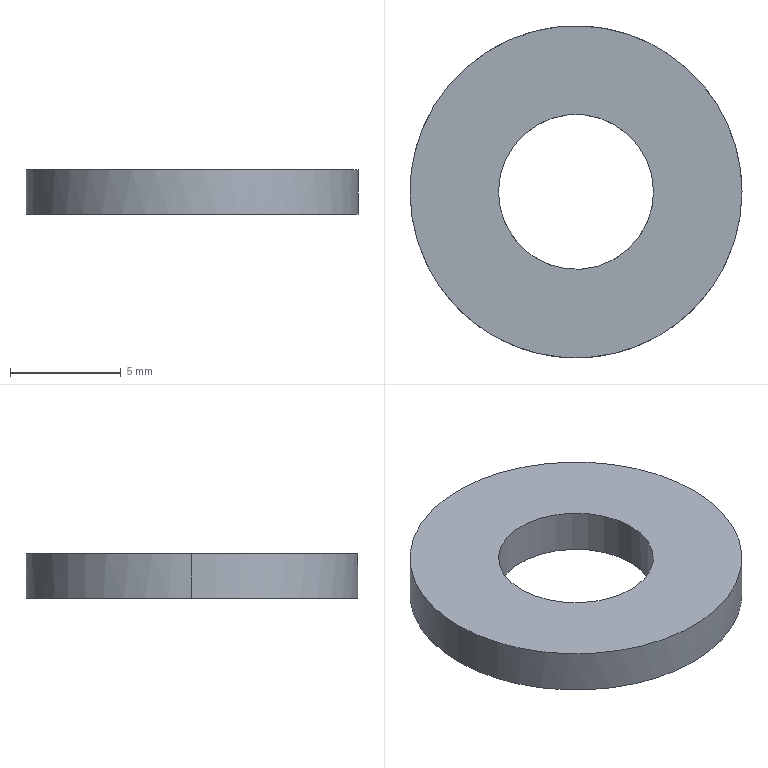Part | STEP file | Positioning_id2198_x_t | 1 solid | 6 faces | box 15 x 15 x 2 mm | volume 276.46 mm3 | cylinder 4 | plane 2 | commonest cylinder face diameters 7 x2 15 x2
STEP:
#1=CARTESIAN_POINT('',(0.,0.,0.));
#2=DIRECTION('',(0.,0.,1.));
#3=DIRECTION('',(1.,0.,0.));
#4=AXIS2_PLACEMENT_3D('',#1,#2,#3);
#5=CARTESIAN_POINT('',(-999.002,416.,33.5));
#6=VERTEX_POINT('',#5);
#7=CARTESIAN_POINT('',(-1006.002,416.,33.5));
#8=VERTEX_POINT('',#7);
#9=CARTESIAN_POINT('',(-1002.502,416.,33.5));
#10=DIRECTION('',(0.,0.,1.));
#11=DIRECTION('',(0.,1.,0.));
#12=AXIS2_PLACEMENT_3D('',#9,#10,#11);
#13=CIRCLE('',#12,3.5);
#14=CARTESIAN_POINT('',(-1002.502,416.,30.5));
#15=DIRECTION('',(0.,0.,-1.));
#16=DIRECTION('',(-1.,0.,0.));
#17=AXIS2_PLACEMENT_3D('',#14,#15,#16);
#18=CYLINDRICAL_SURFACE('',#17,3.5);
#19=CARTESIAN_POINT('',(7.854,-3.));
#20=DIRECTION('',(-1.,0.));
#21=VECTOR('',#20,1.);
#22=LINE('',#19,#21);
#23=(GEOMETRIC_REPRESENTATION_CONTEXT(2)PARAMETRIC_REPRESENTATION_CONTEXT()REPRESENTATION_CONTEXT('',''));
#24=DEFINITIONAL_REPRESENTATION('',(#22),#23);
#25=PCURVE('',#18,#24);
#26=CARTESIAN_POINT('',(-1002.502,416.,33.5));
#27=DIRECTION('',(0.,0.,1.));
#28=DIRECTION('',(-1.,0.,0.));
#29=AXIS2_PLACEMENT_3D('',#26,#27,#28);
#30=PLANE('',#29);
#31=CARTESIAN_POINT('',(0.,0.));
#32=DIRECTION('',(0.,-1.));
#33=AXIS2_PLACEMENT_2D('',#31,#32);
#34=CIRCLE('',#33,3.5);
#35=(GEOMETRIC_REPRESENTATION_CONTEXT(2)PARAMETRIC_REPRESENTATION_CONTEXT()REPRESENTATION_CONTEXT('',''));
#36=DEFINITIONAL_REPRESENTATION('',(#34),#35);
#37=PCURVE('',#30,#36);
#38=SURFACE_CURVE('',#13,(#25,#37),.PCURVE_S1.);
#39=EDGE_CURVE('',#6,#8,#38,.T.);
#40=ORIENTED_EDGE('',*,*,#39,.F.);
#41=CARTESIAN_POINT('',(-999.002,416.,31.5));
#42=VERTEX_POINT('',#41);
#43=CARTESIAN_POINT('',(-999.002,416.,31.5));
#44=DIRECTION('',(0.,0.,1.));
#45=VECTOR('',#44,1.);
#46=LINE('',#43,#45);
#47=CARTESIAN_POINT('',(3.142,-1.));
#48=DIRECTION('',(0.,-1.));
#49=VECTOR('',#48,1.);
#50=LINE('',#47,#49);
#51=(GEOMETRIC_REPRESENTATION_CONTEXT(2)PARAMETRIC_REPRESENTATION_CONTEXT()REPRESENTATION_CONTEXT('',''));
#52=DEFINITIONAL_REPRESENTATION('',(#50),#51);
#53=PCURVE('',#18,#52);
#54=CARTESIAN_POINT('',(-1002.502,416.,30.5));
#55=DIRECTION('',(0.,0.,-1.));
#56=DIRECTION('',(-1.,0.,0.));
#57=AXIS2_PLACEMENT_3D('',#54,#55,#56);
#58=CYLINDRICAL_SURFACE('',#57,3.5);
#59=CARTESIAN_POINT('',(3.142,-1.));
#60=DIRECTION('',(0.,-1.));
#61=VECTOR('',#60,1.);
#62=LINE('',#59,#61);
#63=(GEOMETRIC_REPRESENTATION_CONTEXT(2)PARAMETRIC_REPRESENTATION_CONTEXT()REPRESENTATION_CONTEXT('',''));
#64=DEFINITIONAL_REPRESENTATION('',(#62),#63);
#65=PCURVE('',#58,#64);
#66=SURFACE_CURVE('',#46,(#53,#65),.PCURVE_S1.);
#67=EDGE_CURVE('',#42,#6,#66,.T.);
#68=ORIENTED_EDGE('',*,*,#67,.F.);
#69=CARTESIAN_POINT('',(-1006.002,416.,31.5));
#70=VERTEX_POINT('',#69);
#71=CARTESIAN_POINT('',(-1002.502,416.,31.5));
#72=DIRECTION('',(0.,0.,-1.));
#73=DIRECTION('',(0.,1.,0.));
#74=AXIS2_PLACEMENT_3D('',#71,#72,#73);
#75=CIRCLE('',#74,3.5);
#76=CARTESIAN_POINT('',(-4.712,-1.));
#77=DIRECTION('',(1.,0.));
#78=VECTOR('',#77,1.);
#79=LINE('',#76,#78);
#80=(GEOMETRIC_REPRESENTATION_CONTEXT(2)PARAMETRIC_REPRESENTATION_CONTEXT()REPRESENTATION_CONTEXT('',''));
#81=DEFINITIONAL_REPRESENTATION('',(#79),#80);
#82=PCURVE('',#18,#81);
#83=CARTESIAN_POINT('',(-1002.502,416.,31.5));
#84=DIRECTION('',(0.,0.,-1.));
#85=DIRECTION('',(1.,0.,0.));
#86=AXIS2_PLACEMENT_3D('',#83,#84,#85);
#87=PLANE('',#86);
#88=CARTESIAN_POINT('',(0.,0.));
#89=DIRECTION('',(0.,-1.));
#90=AXIS2_PLACEMENT_2D('',#88,#89);
#91=CIRCLE('',#90,3.5);
#92=(GEOMETRIC_REPRESENTATION_CONTEXT(2)PARAMETRIC_REPRESENTATION_CONTEXT()REPRESENTATION_CONTEXT('',''));
#93=DEFINITIONAL_REPRESENTATION('',(#91),#92);
#94=PCURVE('',#87,#93);
#95=SURFACE_CURVE('',#75,(#82,#94),.PCURVE_S1.);
#96=EDGE_CURVE('',#70,#42,#95,.T.);
#97=ORIENTED_EDGE('',*,*,#96,.F.);
#98=CARTESIAN_POINT('',(-1006.002,416.,31.5));
#99=DIRECTION('',(0.,0.,-1.));
#100=VECTOR('',#99,1.);
#101=LINE('',#98,#100);
#102=CARTESIAN_POINT('',(0.,-1.));
#103=DIRECTION('',(0.,1.));
#104=VECTOR('',#103,1.);
#105=LINE('',#102,#104);
#106=(GEOMETRIC_REPRESENTATION_CONTEXT(2)PARAMETRIC_REPRESENTATION_CONTEXT()REPRESENTATION_CONTEXT('',''));
#107=DEFINITIONAL_REPRESENTATION('',(#105),#106);
#108=PCURVE('',#18,#107);
#109=CARTESIAN_POINT('',(6.283,-1.));
#110=DIRECTION('',(0.,1.));
#111=VECTOR('',#110,1.);
#112=LINE('',#109,#111);
#113=(GEOMETRIC_REPRESENTATION_CONTEXT(2)PARAMETRIC_REPRESENTATION_CONTEXT()REPRESENTATION_CONTEXT('',''));
#114=DEFINITIONAL_REPRESENTATION('',(#112),#113);
#115=PCURVE('',#58,#114);
#116=SURFACE_CURVE('',#101,(#108,#115),.PCURVE_S1.);
#117=EDGE_CURVE('',#8,#70,#116,.T.);
#118=ORIENTED_EDGE('',*,*,#117,.F.);
#119=EDGE_LOOP('',(#40,#68,#97,#118));
#120=FACE_BOUND('',#119,.F.);
#121=ADVANCED_FACE('',(#120),#18,.F.);
#122=CARTESIAN_POINT('',(-1010.002,416.,31.5));
#123=VERTEX_POINT('',#122);
#124=CARTESIAN_POINT('',(-1010.002,416.,33.5));
#125=VERTEX_POINT('',#124);
#126=CARTESIAN_POINT('',(-1010.002,416.,31.5));
#127=DIRECTION('',(0.,0.,1.));
#128=VECTOR('',#127,1.);
#129=LINE('',#126,#128);
#130=CARTESIAN_POINT('',(-1002.502,416.,30.5));
#131=DIRECTION('',(0.,0.,-1.));
#132=DIRECTION('',(-1.,0.,0.));
#133=AXIS2_PLACEMENT_3D('',#130,#131,#132);
#134=CYLINDRICAL_SURFACE('',#133,7.5);
#135=CARTESIAN_POINT('',(6.283,-1.));
#136=DIRECTION('',(0.,-1.));
#137=VECTOR('',#136,1.);
#138=LINE('',#135,#137);
#139=(GEOMETRIC_REPRESENTATION_CONTEXT(2)PARAMETRIC_REPRESENTATION_CONTEXT()REPRESENTATION_CONTEXT('',''));
#140=DEFINITIONAL_REPRESENTATION('',(#138),#139);
#141=PCURVE('',#134,#140);
#142=CARTESIAN_POINT('',(-1002.502,416.,30.5));
#143=DIRECTION('',(0.,0.,-1.));
#144=DIRECTION('',(-1.,0.,0.));
#145=AXIS2_PLACEMENT_3D('',#142,#143,#144);
#146=CYLINDRICAL_SURFACE('',#145,7.5);
#147=CARTESIAN_POINT('',(0.,-1.));
#148=DIRECTION('',(0.,-1.));
#149=VECTOR('',#148,1.);
#150=LINE('',#147,#149);
#151=(GEOMETRIC_REPRESENTATION_CONTEXT(2)PARAMETRIC_REPRESENTATION_CONTEXT()REPRESENTATION_CONTEXT('',''));
#152=DEFINITIONAL_REPRESENTATION('',(#150),#151);
#153=PCURVE('',#146,#152);
#154=SURFACE_CURVE('',#129,(#141,#153),.PCURVE_S1.);
#155=EDGE_CURVE('',#123,#125,#154,.T.);
#156=ORIENTED_EDGE('',*,*,#155,.F.);
#157=CARTESIAN_POINT('',(-1002.502,408.5,31.5));
#158=VERTEX_POINT('',#157);
#159=CARTESIAN_POINT('',(-1002.502,416.,31.5));
#160=DIRECTION('',(0.,0.,-1.));
#161=DIRECTION('',(0.,1.,0.));
#162=AXIS2_PLACEMENT_3D('',#159,#160,#161);
#163=CIRCLE('',#162,7.5);
#164=CARTESIAN_POINT('',(1.571,-1.));
#165=DIRECTION('',(1.,0.));
#166=VECTOR('',#165,1.);
#167=LINE('',#164,#166);
#168=(GEOMETRIC_REPRESENTATION_CONTEXT(2)PARAMETRIC_REPRESENTATION_CONTEXT()REPRESENTATION_CONTEXT('',''));
#169=DEFINITIONAL_REPRESENTATION('',(#167),#168);
#170=PCURVE('',#134,#169);
#171=CARTESIAN_POINT('',(0.,0.));
#172=DIRECTION('',(0.,-1.));
#173=AXIS2_PLACEMENT_2D('',#171,#172);
#174=CIRCLE('',#173,7.5);
#175=(GEOMETRIC_REPRESENTATION_CONTEXT(2)PARAMETRIC_REPRESENTATION_CONTEXT()REPRESENTATION_CONTEXT('',''));
#176=DEFINITIONAL_REPRESENTATION('',(#174),#175);
#177=PCURVE('',#87,#176);
#178=SURFACE_CURVE('',#163,(#170,#177),.PCURVE_S1.);
#179=EDGE_CURVE('',#158,#123,#178,.T.);
#180=ORIENTED_EDGE('',*,*,#179,.F.);
#181=CARTESIAN_POINT('',(-995.002,416.,31.5));
#182=VERTEX_POINT('',#181);
#183=CARTESIAN_POINT('',(-1002.502,416.,31.5));
#184=DIRECTION('',(0.,0.,-1.));
#185=DIRECTION('',(0.,1.,0.));
#186=AXIS2_PLACEMENT_3D('',#183,#184,#185);
#187=CIRCLE('',#186,7.5);
#188=CARTESIAN_POINT('',(1.571,-1.));
#189=DIRECTION('',(1.,0.));
#190=VECTOR('',#189,1.);
#191=LINE('',#188,#190);
#192=(GEOMETRIC_REPRESENTATION_CONTEXT(2)PARAMETRIC_REPRESENTATION_CONTEXT()REPRESENTATION_CONTEXT('',''));
#193=DEFINITIONAL_REPRESENTATION('',(#191),#192);
#194=PCURVE('',#134,#193);
#195=CARTESIAN_POINT('',(0.,0.));
#196=DIRECTION('',(0.,-1.));
#197=AXIS2_PLACEMENT_2D('',#195,#196);
#198=CIRCLE('',#197,7.5);
#199=(GEOMETRIC_REPRESENTATION_CONTEXT(2)PARAMETRIC_REPRESENTATION_CONTEXT()REPRESENTATION_CONTEXT('',''));
#200=DEFINITIONAL_REPRESENTATION('',(#198),#199);
#201=PCURVE('',#87,#200);
#202=SURFACE_CURVE('',#187,(#194,#201),.PCURVE_S1.);
#203=EDGE_CURVE('',#182,#158,#202,.T.);
#204=ORIENTED_EDGE('',*,*,#203,.F.);
#205=CARTESIAN_POINT('',(-995.002,416.,33.5));
#206=VERTEX_POINT('',#205);
#207=CARTESIAN_POINT('',(-995.002,416.,31.5));
#208=DIRECTION('',(0.,0.,-1.));
#209=VECTOR('',#208,1.);
#210=LINE('',#207,#209);
#211=CARTESIAN_POINT('',(3.142,-1.));
#212=DIRECTION('',(0.,1.));
#213=VECTOR('',#212,1.);
#214=LINE('',#211,#213);
#215=(GEOMETRIC_REPRESENTATION_CONTEXT(2)PARAMETRIC_REPRESENTATION_CONTEXT()REPRESENTATION_CONTEXT('',''));
#216=DEFINITIONAL_REPRESENTATION('',(#214),#215);
#217=PCURVE('',#134,#216);
#218=CARTESIAN_POINT('',(3.142,-1.));
#219=DIRECTION('',(0.,1.));
#220=VECTOR('',#219,1.);
#221=LINE('',#218,#220);
#222=(GEOMETRIC_REPRESENTATION_CONTEXT(2)PARAMETRIC_REPRESENTATION_CONTEXT()REPRESENTATION_CONTEXT('',''));
#223=DEFINITIONAL_REPRESENTATION('',(#221),#222);
#224=PCURVE('',#146,#223);
#225=SURFACE_CURVE('',#210,(#217,#224),.PCURVE_S1.);
#226=EDGE_CURVE('',#206,#182,#225,.T.);
#227=ORIENTED_EDGE('',*,*,#226,.F.);
#228=CARTESIAN_POINT('',(-1002.502,416.,33.5));
#229=DIRECTION('',(0.,0.,1.));
#230=DIRECTION('',(0.,1.,0.));
#231=AXIS2_PLACEMENT_3D('',#228,#229,#230);
#232=CIRCLE('',#231,7.5);
#233=CARTESIAN_POINT('',(7.854,-3.));
#234=DIRECTION('',(-1.,0.));
#235=VECTOR('',#234,1.);
#236=LINE('',#233,#235);
#237=(GEOMETRIC_REPRESENTATION_CONTEXT(2)PARAMETRIC_REPRESENTATION_CONTEXT()REPRESENTATION_CONTEXT('',''));
#238=DEFINITIONAL_REPRESENTATION('',(#236),#237);
#239=PCURVE('',#134,#238);
#240=CARTESIAN_POINT('',(0.,0.));
#241=DIRECTION('',(0.,-1.));
#242=AXIS2_PLACEMENT_2D('',#240,#241);
#243=CIRCLE('',#242,7.5);
#244=(GEOMETRIC_REPRESENTATION_CONTEXT(2)PARAMETRIC_REPRESENTATION_CONTEXT()REPRESENTATION_CONTEXT('',''));
#245=DEFINITIONAL_REPRESENTATION('',(#243),#244);
#246=PCURVE('',#30,#245);
#247=SURFACE_CURVE('',#232,(#239,#246),.PCURVE_S1.);
#248=EDGE_CURVE('',#125,#206,#247,.T.);
#249=ORIENTED_EDGE('',*,*,#248,.F.);
#250=EDGE_LOOP('',(#156,#180,#204,#227,#249));
#251=FACE_BOUND('',#250,.T.);
#252=ADVANCED_FACE('',(#251),#134,.T.);
#253=CARTESIAN_POINT('',(-1002.502,412.5,31.5));
#254=VERTEX_POINT('',#253);
#255=CARTESIAN_POINT('',(-999.002,416.,31.5));
#256=CARTESIAN_POINT('',(-999.002,412.5,31.5));
#257=CARTESIAN_POINT('',(-1002.502,412.5,31.5));
#258=(BOUNDED_CURVE()B_SPLINE_CURVE(2,(#255,#256,#257),.UNSPECIFIED.,.F.,.F.)B_SPLINE_CURVE_WITH_KNOTS((3,3),(0.,1.),.PIECEWISE_BEZIER_KNOTS.)CURVE()GEOMETRIC_REPRESENTATION_ITEM()RATIONAL_B_SPLINE_CURVE((1.,0.7071,1.))REPRESENTATION_ITEM(''));
#259=CARTESIAN_POINT('',(3.5,0.));
#260=CARTESIAN_POINT('',(3.5,3.5));
#261=CARTESIAN_POINT('',(0.,3.5));
#262=(BOUNDED_CURVE()B_SPLINE_CURVE(2,(#259,#260,#261),.UNSPECIFIED.,.F.,.F.)B_SPLINE_CURVE_WITH_KNOTS((3,3),(0.,1.),.PIECEWISE_BEZIER_KNOTS.)CURVE()GEOMETRIC_REPRESENTATION_ITEM()RATIONAL_B_SPLINE_CURVE((1.,0.7071,1.))REPRESENTATION_ITEM(''));
#263=(GEOMETRIC_REPRESENTATION_CONTEXT(2)PARAMETRIC_REPRESENTATION_CONTEXT()REPRESENTATION_CONTEXT('',''));
#264=DEFINITIONAL_REPRESENTATION('',(#262),#263);
#265=PCURVE('',#87,#264);
#266=CARTESIAN_POINT('',(3.142,-1.));
#267=CARTESIAN_POINT('',(3.163,-1.));
#268=CARTESIAN_POINT('',(3.206,-1.));
#269=CARTESIAN_POINT('',(3.273,-1.));
#270=CARTESIAN_POINT('',(3.342,-1.));
#271=CARTESIAN_POINT('',(3.411,-1.));
#272=CARTESIAN_POINT('',(3.482,-1.));
#273=CARTESIAN_POINT('',(3.555,-1.));
#274=CARTESIAN_POINT('',(3.628,-1.));
#275=CARTESIAN_POINT('',(3.702,-1.));
#276=CARTESIAN_POINT('',(3.777,-1.));
#277=CARTESIAN_POINT('',(3.852,-1.));
#278=CARTESIAN_POINT('',(3.927,-1.));
#279=CARTESIAN_POINT('',(4.002,-1.));
#280=CARTESIAN_POINT('',(4.077,-1.));
#281=CARTESIAN_POINT('',(4.152,-1.));
#282=CARTESIAN_POINT('',(4.226,-1.));
#283=CARTESIAN_POINT('',(4.299,-1.));
#284=CARTESIAN_POINT('',(4.372,-1.));
#285=CARTESIAN_POINT('',(4.443,-1.));
#286=CARTESIAN_POINT('',(4.512,-1.));
#287=CARTESIAN_POINT('',(4.581,-1.));
#288=CARTESIAN_POINT('',(4.648,-1.));
#289=CARTESIAN_POINT('',(4.691,-1.));
#290=CARTESIAN_POINT('',(4.712,-1.));
#291=B_SPLINE_CURVE_WITH_KNOTS('',3,(#266,#267,#268,#269,#270,#271,#272,#273,#274,#275,#276,#277,#278,#279,#280,#281,#282,#283,#284,#285,#286,#287,#288,#289,#290),.UNSPECIFIED.,.F.,.F.,(4,1,1,1,1,1,1,1,1,1,1,1,1,1,1,1,1,1,1,1,1,1,4),(0.,0.04545,0.09091,0.1364,0.1818,0.2273,0.2727,0.3182,0.3636,0.4091,0.4545,0.5,0.5455,0.5909,0.6364,0.6818,0.7273,0.7727,0.8182,0.8636,0.9091,0.9545,1.),.QUASI_UNIFORM_KNOTS.);
#292=(GEOMETRIC_REPRESENTATION_CONTEXT(2)PARAMETRIC_REPRESENTATION_CONTEXT()REPRESENTATION_CONTEXT('',''));
#293=DEFINITIONAL_REPRESENTATION('',(#291),#292);
#294=PCURVE('',#58,#293);
#295=SURFACE_CURVE('',#258,(#265,#294),.PCURVE_S1.);
#296=EDGE_CURVE('',#42,#254,#295,.T.);
#297=ORIENTED_EDGE('',*,*,#296,.F.);
#298=ORIENTED_EDGE('',*,*,#96,.F.);
#299=CARTESIAN_POINT('',(-1002.502,412.5,31.5));
#300=CARTESIAN_POINT('',(-1006.002,412.5,31.5));
#301=CARTESIAN_POINT('',(-1006.002,416.,31.5));
#302=(BOUNDED_CURVE()B_SPLINE_CURVE(2,(#299,#300,#301),.UNSPECIFIED.,.F.,.F.)B_SPLINE_CURVE_WITH_KNOTS((3,3),(0.,1.),.PIECEWISE_BEZIER_KNOTS.)CURVE()GEOMETRIC_REPRESENTATION_ITEM()RATIONAL_B_SPLINE_CURVE((1.,0.7071,1.))REPRESENTATION_ITEM(''));
#303=CARTESIAN_POINT('',(0.,3.5));
#304=CARTESIAN_POINT('',(-3.5,3.5));
#305=CARTESIAN_POINT('',(-3.5,0.));
#306=(BOUNDED_CURVE()B_SPLINE_CURVE(2,(#303,#304,#305),.UNSPECIFIED.,.F.,.F.)B_SPLINE_CURVE_WITH_KNOTS((3,3),(0.,1.),.PIECEWISE_BEZIER_KNOTS.)CURVE()GEOMETRIC_REPRESENTATION_ITEM()RATIONAL_B_SPLINE_CURVE((1.,0.7071,1.))REPRESENTATION_ITEM(''));
#307=(GEOMETRIC_REPRESENTATION_CONTEXT(2)PARAMETRIC_REPRESENTATION_CONTEXT()REPRESENTATION_CONTEXT('',''));
#308=DEFINITIONAL_REPRESENTATION('',(#306),#307);
#309=PCURVE('',#87,#308);
#310=CARTESIAN_POINT('',(4.712,-1.));
#311=CARTESIAN_POINT('',(4.734,-1.));
#312=CARTESIAN_POINT('',(4.777,-1.));
#313=CARTESIAN_POINT('',(4.844,-1.));
#314=CARTESIAN_POINT('',(4.912,-1.));
#315=CARTESIAN_POINT('',(4.982,-1.));
#316=CARTESIAN_POINT('',(5.053,-1.));
#317=CARTESIAN_POINT('',(5.125,-1.));
#318=CARTESIAN_POINT('',(5.199,-1.));
#319=CARTESIAN_POINT('',(5.273,-1.));
#320=CARTESIAN_POINT('',(5.347,-1.));
#321=CARTESIAN_POINT('',(5.422,-1.));
#322=CARTESIAN_POINT('',(5.498,-1.));
#323=CARTESIAN_POINT('',(5.573,-1.));
#324=CARTESIAN_POINT('',(5.648,-1.));
#325=CARTESIAN_POINT('',(5.723,-1.));
#326=CARTESIAN_POINT('',(5.797,-1.));
#327=CARTESIAN_POINT('',(5.87,-1.));
#328=CARTESIAN_POINT('',(5.942,-1.));
#329=CARTESIAN_POINT('',(6.013,-1.));
#330=CARTESIAN_POINT('',(6.083,-1.));
#331=CARTESIAN_POINT('',(6.152,-1.));
#332=CARTESIAN_POINT('',(6.218,-1.));
#333=CARTESIAN_POINT('',(6.262,-1.));
#334=CARTESIAN_POINT('',(6.283,-1.));
#335=B_SPLINE_CURVE_WITH_KNOTS('',3,(#310,#311,#312,#313,#314,#315,#316,#317,#318,#319,#320,#321,#322,#323,#324,#325,#326,#327,#328,#329,#330,#331,#332,#333,#334),.UNSPECIFIED.,.F.,.F.,(4,1,1,1,1,1,1,1,1,1,1,1,1,1,1,1,1,1,1,1,1,1,4),(0.,0.04545,0.09091,0.1364,0.1818,0.2273,0.2727,0.3182,0.3636,0.4091,0.4545,0.5,0.5455,0.5909,0.6364,0.6818,0.7273,0.7727,0.8182,0.8636,0.9091,0.9545,1.),.QUASI_UNIFORM_KNOTS.);
#336=(GEOMETRIC_REPRESENTATION_CONTEXT(2)PARAMETRIC_REPRESENTATION_CONTEXT()REPRESENTATION_CONTEXT('',''));
#337=DEFINITIONAL_REPRESENTATION('',(#335),#336);
#338=PCURVE('',#58,#337);
#339=SURFACE_CURVE('',#302,(#309,#338),.PCURVE_S1.);
#340=EDGE_CURVE('',#254,#70,#339,.T.);
#341=ORIENTED_EDGE('',*,*,#340,.F.);
#342=EDGE_LOOP('',(#297,#298,#341));
#343=FACE_BOUND('',#342,.T.);
#344=ORIENTED_EDGE('',*,*,#203,.T.);
#345=ORIENTED_EDGE('',*,*,#179,.T.);
#346=CARTESIAN_POINT('',(-1010.002,416.,31.5));
#347=CARTESIAN_POINT('',(-1010.002,423.5,31.5));
#348=CARTESIAN_POINT('',(-1002.502,427.25,31.5));
#349=CARTESIAN_POINT('',(-995.002,423.5,31.5));
#350=CARTESIAN_POINT('',(-995.002,416.,31.5));
#351=(BOUNDED_CURVE()B_SPLINE_CURVE(4,(#346,#347,#348,#349,#350),.UNSPECIFIED.,.F.,.F.)B_SPLINE_CURVE_WITH_KNOTS((5,5),(0.,1.),.PIECEWISE_BEZIER_KNOTS.)CURVE()GEOMETRIC_REPRESENTATION_ITEM()RATIONAL_B_SPLINE_CURVE((1.,0.7071,0.6667,0.7071,1.))REPRESENTATION_ITEM(''));
#352=CARTESIAN_POINT('',(-7.5,0.));
#353=CARTESIAN_POINT('',(-7.5,-7.5));
#354=CARTESIAN_POINT('',(0.,-11.25));
#355=CARTESIAN_POINT('',(7.5,-7.5));
#356=CARTESIAN_POINT('',(7.5,0.));
#357=(BOUNDED_CURVE()B_SPLINE_CURVE(4,(#352,#353,#354,#355,#356),.UNSPECIFIED.,.F.,.F.)B_SPLINE_CURVE_WITH_KNOTS((5,5),(0.,1.),.PIECEWISE_BEZIER_KNOTS.)CURVE()GEOMETRIC_REPRESENTATION_ITEM()RATIONAL_B_SPLINE_CURVE((1.,0.7071,0.6667,0.7071,1.))REPRESENTATION_ITEM(''));
#358=(GEOMETRIC_REPRESENTATION_CONTEXT(2)PARAMETRIC_REPRESENTATION_CONTEXT()REPRESENTATION_CONTEXT('',''));
#359=DEFINITIONAL_REPRESENTATION('',(#357),#358);
#360=PCURVE('',#87,#359);
#361=CARTESIAN_POINT('',(0.,-1.));
#362=CARTESIAN_POINT('',(0.04285,-1.));
#363=CARTESIAN_POINT('',(0.1297,-1.));
#364=CARTESIAN_POINT('',(0.2633,-1.));
#365=CARTESIAN_POINT('',(0.3999,-1.));
#366=CARTESIAN_POINT('',(0.5394,-1.));
#367=CARTESIAN_POINT('',(0.6816,-1.));
#368=CARTESIAN_POINT('',(0.8261,-1.));
#369=CARTESIAN_POINT('',(0.9725,-1.));
#370=CARTESIAN_POINT('',(1.121,-1.));
#371=CARTESIAN_POINT('',(1.27,-1.));
#372=CARTESIAN_POINT('',(1.42,-1.));
#373=CARTESIAN_POINT('',(1.571,-1.));
#374=CARTESIAN_POINT('',(1.721,-1.));
#375=CARTESIAN_POINT('',(1.872,-1.));
#376=CARTESIAN_POINT('',(2.021,-1.));
#377=CARTESIAN_POINT('',(2.169,-1.));
#378=CARTESIAN_POINT('',(2.316,-1.));
#379=CARTESIAN_POINT('',(2.46,-1.));
#380=CARTESIAN_POINT('',(2.602,-1.));
#381=CARTESIAN_POINT('',(2.742,-1.));
#382=CARTESIAN_POINT('',(2.878,-1.));
#383=CARTESIAN_POINT('',(3.012,-1.));
#384=CARTESIAN_POINT('',(3.099,-1.));
#385=CARTESIAN_POINT('',(3.142,-1.));
#386=B_SPLINE_CURVE_WITH_KNOTS('',3,(#361,#362,#363,#364,#365,#366,#367,#368,#369,#370,#371,#372,#373,#374,#375,#376,#377,#378,#379,#380,#381,#382,#383,#384,#385),.UNSPECIFIED.,.F.,.F.,(4,1,1,1,1,1,1,1,1,1,1,1,1,1,1,1,1,1,1,1,1,1,4),(0.,0.04545,0.09091,0.1364,0.1818,0.2273,0.2727,0.3182,0.3636,0.4091,0.4545,0.5,0.5455,0.5909,0.6364,0.6818,0.7273,0.7727,0.8182,0.8636,0.9091,0.9545,1.),.QUASI_UNIFORM_KNOTS.);
#387=(GEOMETRIC_REPRESENTATION_CONTEXT(2)PARAMETRIC_REPRESENTATION_CONTEXT()REPRESENTATION_CONTEXT('',''));
#388=DEFINITIONAL_REPRESENTATION('',(#386),#387);
#389=PCURVE('',#146,#388);
#390=SURFACE_CURVE('',#351,(#360,#389),.PCURVE_S1.);
#391=EDGE_CURVE('',#123,#182,#390,.T.);
#392=ORIENTED_EDGE('',*,*,#391,.T.);
#393=EDGE_LOOP('',(#344,#345,#392));
#394=FACE_BOUND('',#393,.T.);
#395=ADVANCED_FACE('',(#343,#394),#87,.T.);
#396=ORIENTED_EDGE('',*,*,#39,.F.);
#397=CARTESIAN_POINT('',(-1006.002,416.,33.5));
#398=CARTESIAN_POINT('',(-1006.002,412.5,33.5));
#399=CARTESIAN_POINT('',(-1002.502,410.75,33.5));
#400=CARTESIAN_POINT('',(-999.002,412.5,33.5));
#401=CARTESIAN_POINT('',(-999.002,416.,33.5));
#402=(BOUNDED_CURVE()B_SPLINE_CURVE(4,(#397,#398,#399,#400,#401),.UNSPECIFIED.,.F.,.F.)B_SPLINE_CURVE_WITH_KNOTS((5,5),(0.,1.),.PIECEWISE_BEZIER_KNOTS.)CURVE()GEOMETRIC_REPRESENTATION_ITEM()RATIONAL_B_SPLINE_CURVE((1.,0.7071,0.6667,0.7071,1.))REPRESENTATION_ITEM(''));
#403=CARTESIAN_POINT('',(3.5,0.));
#404=CARTESIAN_POINT('',(3.5,3.5));
#405=CARTESIAN_POINT('',(0.,5.25));
#406=CARTESIAN_POINT('',(-3.5,3.5));
#407=CARTESIAN_POINT('',(-3.5,0.));
#408=(BOUNDED_CURVE()B_SPLINE_CURVE(4,(#403,#404,#405,#406,#407),.UNSPECIFIED.,.F.,.F.)B_SPLINE_CURVE_WITH_KNOTS((5,5),(0.,1.),.PIECEWISE_BEZIER_KNOTS.)CURVE()GEOMETRIC_REPRESENTATION_ITEM()RATIONAL_B_SPLINE_CURVE((1.,0.7071,0.6667,0.7071,1.))REPRESENTATION_ITEM(''));
#409=(GEOMETRIC_REPRESENTATION_CONTEXT(2)PARAMETRIC_REPRESENTATION_CONTEXT()REPRESENTATION_CONTEXT('',''));
#410=DEFINITIONAL_REPRESENTATION('',(#408),#409);
#411=PCURVE('',#30,#410);
#412=CARTESIAN_POINT('',(6.283,-3.));
#413=CARTESIAN_POINT('',(6.24,-3.));
#414=CARTESIAN_POINT('',(6.153,-3.));
#415=CARTESIAN_POINT('',(6.02,-3.));
#416=CARTESIAN_POINT('',(5.883,-3.));
#417=CARTESIAN_POINT('',(5.744,-3.));
#418=CARTESIAN_POINT('',(5.602,-3.));
#419=CARTESIAN_POINT('',(5.457,-3.));
#420=CARTESIAN_POINT('',(5.311,-3.));
#421=CARTESIAN_POINT('',(5.163,-3.));
#422=CARTESIAN_POINT('',(5.013,-3.));
#423=CARTESIAN_POINT('',(4.863,-3.));
#424=CARTESIAN_POINT('',(4.712,-3.));
#425=CARTESIAN_POINT('',(4.562,-3.));
#426=CARTESIAN_POINT('',(4.412,-3.));
#427=CARTESIAN_POINT('',(4.262,-3.));
#428=CARTESIAN_POINT('',(4.114,-3.));
#429=CARTESIAN_POINT('',(3.968,-3.));
#430=CARTESIAN_POINT('',(3.823,-3.));
#431=CARTESIAN_POINT('',(3.681,-3.));
#432=CARTESIAN_POINT('',(3.542,-3.));
#433=CARTESIAN_POINT('',(3.405,-3.));
#434=CARTESIAN_POINT('',(3.271,-3.));
#435=CARTESIAN_POINT('',(3.184,-3.));
#436=CARTESIAN_POINT('',(3.142,-3.));
#437=B_SPLINE_CURVE_WITH_KNOTS('',3,(#412,#413,#414,#415,#416,#417,#418,#419,#420,#421,#422,#423,#424,#425,#426,#427,#428,#429,#430,#431,#432,#433,#434,#435,#436),.UNSPECIFIED.,.F.,.F.,(4,1,1,1,1,1,1,1,1,1,1,1,1,1,1,1,1,1,1,1,1,1,4),(0.,0.04545,0.09091,0.1364,0.1818,0.2273,0.2727,0.3182,0.3636,0.4091,0.4545,0.5,0.5455,0.5909,0.6364,0.6818,0.7273,0.7727,0.8182,0.8636,0.9091,0.9545,1.),.QUASI_UNIFORM_KNOTS.);
#438=(GEOMETRIC_REPRESENTATION_CONTEXT(2)PARAMETRIC_REPRESENTATION_CONTEXT()REPRESENTATION_CONTEXT('',''));
#439=DEFINITIONAL_REPRESENTATION('',(#437),#438);
#440=PCURVE('',#58,#439);
#441=SURFACE_CURVE('',#402,(#411,#440),.PCURVE_S1.);
#442=EDGE_CURVE('',#8,#6,#441,.T.);
#443=ORIENTED_EDGE('',*,*,#442,.F.);
#444=EDGE_LOOP('',(#396,#443));
#445=FACE_BOUND('',#444,.T.);
#446=CARTESIAN_POINT('',(-995.002,416.,33.5));
#447=CARTESIAN_POINT('',(-995.002,423.5,33.5));
#448=CARTESIAN_POINT('',(-1002.502,427.25,33.5));
#449=CARTESIAN_POINT('',(-1010.002,423.5,33.5));
#450=CARTESIAN_POINT('',(-1010.002,416.,33.5));
#451=(BOUNDED_CURVE()B_SPLINE_CURVE(4,(#446,#447,#448,#449,#450),.UNSPECIFIED.,.F.,.F.)B_SPLINE_CURVE_WITH_KNOTS((5,5),(0.,1.),.PIECEWISE_BEZIER_KNOTS.)CURVE()GEOMETRIC_REPRESENTATION_ITEM()RATIONAL_B_SPLINE_CURVE((1.,0.7071,0.6667,0.7071,1.))REPRESENTATION_ITEM(''));
#452=CARTESIAN_POINT('',(-7.5,0.));
#453=CARTESIAN_POINT('',(-7.5,-7.5));
#454=CARTESIAN_POINT('',(0.,-11.25));
#455=CARTESIAN_POINT('',(7.5,-7.5));
#456=CARTESIAN_POINT('',(7.5,0.));
#457=(BOUNDED_CURVE()B_SPLINE_CURVE(4,(#452,#453,#454,#455,#456),.UNSPECIFIED.,.F.,.F.)B_SPLINE_CURVE_WITH_KNOTS((5,5),(0.,1.),.PIECEWISE_BEZIER_KNOTS.)CURVE()GEOMETRIC_REPRESENTATION_ITEM()RATIONAL_B_SPLINE_CURVE((1.,0.7071,0.6667,0.7071,1.))REPRESENTATION_ITEM(''));
#458=(GEOMETRIC_REPRESENTATION_CONTEXT(2)PARAMETRIC_REPRESENTATION_CONTEXT()REPRESENTATION_CONTEXT('',''));
#459=DEFINITIONAL_REPRESENTATION('',(#457),#458);
#460=PCURVE('',#30,#459);
#461=CARTESIAN_POINT('',(3.142,-3.));
#462=CARTESIAN_POINT('',(3.099,-3.));
#463=CARTESIAN_POINT('',(3.012,-3.));
#464=CARTESIAN_POINT('',(2.878,-3.));
#465=CARTESIAN_POINT('',(2.742,-3.));
#466=CARTESIAN_POINT('',(2.602,-3.));
#467=CARTESIAN_POINT('',(2.46,-3.));
#468=CARTESIAN_POINT('',(2.316,-3.));
#469=CARTESIAN_POINT('',(2.169,-3.));
#470=CARTESIAN_POINT('',(2.021,-3.));
#471=CARTESIAN_POINT('',(1.872,-3.));
#472=CARTESIAN_POINT('',(1.721,-3.));
#473=CARTESIAN_POINT('',(1.571,-3.));
#474=CARTESIAN_POINT('',(1.42,-3.));
#475=CARTESIAN_POINT('',(1.27,-3.));
#476=CARTESIAN_POINT('',(1.121,-3.));
#477=CARTESIAN_POINT('',(0.9725,-3.));
#478=CARTESIAN_POINT('',(0.8261,-3.));
#479=CARTESIAN_POINT('',(0.6816,-3.));
#480=CARTESIAN_POINT('',(0.5394,-3.));
#481=CARTESIAN_POINT('',(0.3999,-3.));
#482=CARTESIAN_POINT('',(0.2633,-3.));
#483=CARTESIAN_POINT('',(0.1297,-3.));
#484=CARTESIAN_POINT('',(0.04285,-3.));
#485=CARTESIAN_POINT('',(0.,-3.));
#486=B_SPLINE_CURVE_WITH_KNOTS('',3,(#461,#462,#463,#464,#465,#466,#467,#468,#469,#470,#471,#472,#473,#474,#475,#476,#477,#478,#479,#480,#481,#482,#483,#484,#485),.UNSPECIFIED.,.F.,.F.,(4,1,1,1,1,1,1,1,1,1,1,1,1,1,1,1,1,1,1,1,1,1,4),(0.,0.04545,0.09091,0.1364,0.1818,0.2273,0.2727,0.3182,0.3636,0.4091,0.4545,0.5,0.5455,0.5909,0.6364,0.6818,0.7273,0.7727,0.8182,0.8636,0.9091,0.9545,1.),.QUASI_UNIFORM_KNOTS.);
#487=(GEOMETRIC_REPRESENTATION_CONTEXT(2)PARAMETRIC_REPRESENTATION_CONTEXT()REPRESENTATION_CONTEXT('',''));
#488=DEFINITIONAL_REPRESENTATION('',(#486),#487);
#489=PCURVE('',#146,#488);
#490=SURFACE_CURVE('',#451,(#460,#489),.PCURVE_S1.);
#491=EDGE_CURVE('',#206,#125,#490,.T.);
#492=ORIENTED_EDGE('',*,*,#491,.T.);
#493=ORIENTED_EDGE('',*,*,#248,.T.);
#494=EDGE_LOOP('',(#492,#493));
#495=FACE_BOUND('',#494,.T.);
#496=ADVANCED_FACE('',(#445,#495),#30,.T.);
#497=ORIENTED_EDGE('',*,*,#391,.F.);
#498=ORIENTED_EDGE('',*,*,#155,.T.);
#499=ORIENTED_EDGE('',*,*,#491,.F.);
#500=ORIENTED_EDGE('',*,*,#226,.T.);
#501=EDGE_LOOP('',(#497,#498,#499,#500));
#502=FACE_BOUND('',#501,.T.);
#503=ADVANCED_FACE('',(#502),#146,.T.);
#504=ORIENTED_EDGE('',*,*,#67,.T.);
#505=ORIENTED_EDGE('',*,*,#442,.F.);
#506=ORIENTED_EDGE('',*,*,#117,.T.);
#507=ORIENTED_EDGE('',*,*,#340,.F.);
#508=ORIENTED_EDGE('',*,*,#296,.F.);
#509=EDGE_LOOP('',(#504,#505,#506,#507,#508));
#510=FACE_BOUND('',#509,.F.);
#511=ADVANCED_FACE('',(#510),#58,.F.);
#512=CLOSED_SHELL('',(#121,#252,#395,#496,#503,#511));
#513=MANIFOLD_SOLID_BREP('',#512);
#514=(LENGTH_UNIT()NAMED_UNIT(*)SI_UNIT(.MILLI.,.METRE.));
#515=UNCERTAINTY_MEASURE_WITH_UNIT(LENGTH_MEASURE(0.0000001),#514,'','');
#516=(NAMED_UNIT(*)PLANE_ANGLE_UNIT()SI_UNIT($,.RADIAN.));
#517=(NAMED_UNIT(*)SI_UNIT($,.STERADIAN.)SOLID_ANGLE_UNIT());
#518=(GEOMETRIC_REPRESENTATION_CONTEXT(3)GLOBAL_UNCERTAINTY_ASSIGNED_CONTEXT((#515))GLOBAL_UNIT_ASSIGNED_CONTEXT((#514,#516,#517))REPRESENTATION_CONTEXT('',''));
#519=ADVANCED_BREP_SHAPE_REPRESENTATION('',(#4,#513),#518);